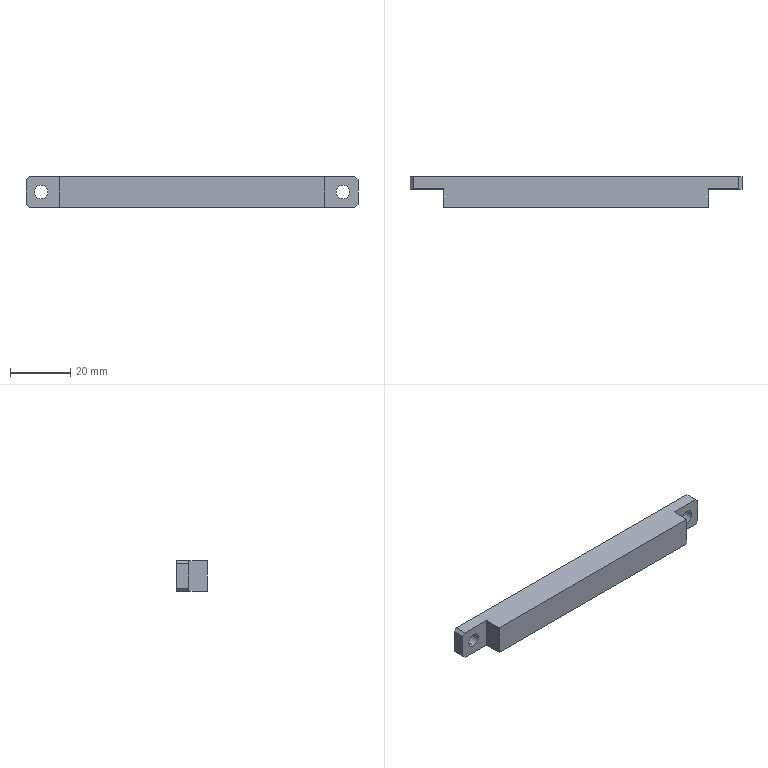Part | STEP file | 08-10 stop block | 1 solid | 18 faces | box 110 x 10 x 10 mm | volume 9545 mm3 | plane 14 | cylinder 4 | commonest cylinder face diameters 4.5 x4
STEP:
#1=CARTESIAN_POINT('',(-50.,-1.5,2.75));
#2=VERTEX_POINT('',#1);
#3=CARTESIAN_POINT('',(-50.,-1.5,7.25));
#4=VERTEX_POINT('',#3);
#5=CARTESIAN_POINT('',(-50.,-1.5,5.));
#6=DIRECTION('',(0.,1.,0.));
#7=DIRECTION('',(-1.,0.,0.));
#8=AXIS2_PLACEMENT_3D('',#5,#6,#7);
#9=CIRCLE('',#8,2.25);
#10=EDGE_CURVE('',#2,#4,#9,.T.);
#11=ORIENTED_EDGE('',*,*,#10,.F.);
#12=CARTESIAN_POINT('',(-50.,2.5,2.75));
#13=VERTEX_POINT('',#12);
#14=CARTESIAN_POINT('',(-50.,7.5,2.75));
#15=DIRECTION('',(0.,1.,0.));
#16=VECTOR('',#15,1000.);
#17=LINE('',#14,#16);
#18=EDGE_CURVE('',#2,#13,#17,.T.);
#19=ORIENTED_EDGE('',*,*,#18,.T.);
#20=CARTESIAN_POINT('',(-50.,2.5,7.25));
#21=VERTEX_POINT('',#20);
#22=CARTESIAN_POINT('',(-50.,2.5,5.));
#23=DIRECTION('',(0.,1.,0.));
#24=DIRECTION('',(0.,0.,-1.));
#25=AXIS2_PLACEMENT_3D('',#22,#23,#24);
#26=CIRCLE('',#25,2.25);
#27=EDGE_CURVE('',#13,#21,#26,.T.);
#28=ORIENTED_EDGE('',*,*,#27,.T.);
#29=CARTESIAN_POINT('',(-50.,7.5,7.25));
#30=DIRECTION('',(0.,1.,0.));
#31=VECTOR('',#30,1000.);
#32=LINE('',#29,#31);
#33=EDGE_CURVE('',#4,#21,#32,.T.);
#34=ORIENTED_EDGE('',*,*,#33,.F.);
#35=EDGE_LOOP('',(#11,#19,#28,#34));
#36=FACE_OUTER_BOUND('',#35,.T.);
#37=CARTESIAN_POINT('',(-50.,7.5,5.));
#38=DIRECTION('',(0.,1.,0.));
#39=DIRECTION('',(0.,0.,1.));
#40=AXIS2_PLACEMENT_3D('',#37,#38,#39);
#41=CYLINDRICAL_SURFACE('',#40,2.25);
#42=ADVANCED_FACE('',(#36),#41,.F.);
#43=CARTESIAN_POINT('',(50.,-1.5,2.75));
#44=VERTEX_POINT('',#43);
#45=CARTESIAN_POINT('',(50.,-1.5,7.25));
#46=VERTEX_POINT('',#45);
#47=CARTESIAN_POINT('',(50.,-1.5,5.));
#48=DIRECTION('',(0.,1.,0.));
#49=DIRECTION('',(-1.,0.,0.));
#50=AXIS2_PLACEMENT_3D('',#47,#48,#49);
#51=CIRCLE('',#50,2.25);
#52=EDGE_CURVE('',#44,#46,#51,.T.);
#53=ORIENTED_EDGE('',*,*,#52,.F.);
#54=CARTESIAN_POINT('',(50.,2.5,2.75));
#55=VERTEX_POINT('',#54);
#56=CARTESIAN_POINT('',(50.,7.5,2.75));
#57=DIRECTION('',(0.,1.,0.));
#58=VECTOR('',#57,1000.);
#59=LINE('',#56,#58);
#60=EDGE_CURVE('',#44,#55,#59,.T.);
#61=ORIENTED_EDGE('',*,*,#60,.T.);
#62=CARTESIAN_POINT('',(50.,2.5,7.25));
#63=VERTEX_POINT('',#62);
#64=CARTESIAN_POINT('',(50.,2.5,5.));
#65=DIRECTION('',(0.,1.,0.));
#66=DIRECTION('',(0.,0.,-1.));
#67=AXIS2_PLACEMENT_3D('',#64,#65,#66);
#68=CIRCLE('',#67,2.25);
#69=EDGE_CURVE('',#55,#63,#68,.T.);
#70=ORIENTED_EDGE('',*,*,#69,.T.);
#71=CARTESIAN_POINT('',(50.,7.5,7.25));
#72=DIRECTION('',(0.,1.,0.));
#73=VECTOR('',#72,1000.);
#74=LINE('',#71,#73);
#75=EDGE_CURVE('',#46,#63,#74,.T.);
#76=ORIENTED_EDGE('',*,*,#75,.F.);
#77=EDGE_LOOP('',(#53,#61,#70,#76));
#78=FACE_OUTER_BOUND('',#77,.T.);
#79=CARTESIAN_POINT('',(50.,7.5,5.));
#80=DIRECTION('',(0.,1.,0.));
#81=DIRECTION('',(0.,0.,1.));
#82=AXIS2_PLACEMENT_3D('',#79,#80,#81);
#83=CYLINDRICAL_SURFACE('',#82,2.25);
#84=ADVANCED_FACE('',(#78),#83,.F.);
#85=CARTESIAN_POINT('',(55.,-1.5,1.));
#86=VERTEX_POINT('',#85);
#87=CARTESIAN_POINT('',(55.,2.5,1.));
#88=VERTEX_POINT('',#87);
#89=CARTESIAN_POINT('',(55.,7.5,1.));
#90=DIRECTION('',(0.,1.,0.));
#91=VECTOR('',#90,1000.);
#92=LINE('',#89,#91);
#93=EDGE_CURVE('',#86,#88,#92,.T.);
#94=ORIENTED_EDGE('',*,*,#93,.T.);
#95=CARTESIAN_POINT('',(55.,2.5,9.));
#96=VERTEX_POINT('',#95);
#97=CARTESIAN_POINT('',(55.,2.5,10.));
#98=DIRECTION('',(0.,0.,1.));
#99=VECTOR('',#98,1000.);
#100=LINE('',#97,#99);
#101=EDGE_CURVE('',#88,#96,#100,.T.);
#102=ORIENTED_EDGE('',*,*,#101,.T.);
#103=CARTESIAN_POINT('',(55.,-1.5,9.));
#104=VERTEX_POINT('',#103);
#105=CARTESIAN_POINT('',(55.,-1.5,9.));
#106=DIRECTION('',(0.,-1.,0.));
#107=VECTOR('',#106,1000.);
#108=LINE('',#105,#107);
#109=EDGE_CURVE('',#96,#104,#108,.T.);
#110=ORIENTED_EDGE('',*,*,#109,.T.);
#111=CARTESIAN_POINT('',(55.,-1.5,0.));
#112=DIRECTION('',(0.,0.,1.));
#113=VECTOR('',#112,1000.);
#114=LINE('',#111,#113);
#115=EDGE_CURVE('',#86,#104,#114,.T.);
#116=ORIENTED_EDGE('',*,*,#115,.F.);
#117=EDGE_LOOP('',(#94,#102,#110,#116));
#118=FACE_OUTER_BOUND('',#117,.T.);
#119=CARTESIAN_POINT('',(55.,7.5,10.));
#120=DIRECTION('',(-1.,0.,0.));
#121=DIRECTION('',(0.,0.,1.));
#122=AXIS2_PLACEMENT_3D('',#119,#120,#121);
#123=PLANE('',#122);
#124=ADVANCED_FACE('',(#118),#123,.F.);
#125=CARTESIAN_POINT('',(-55.,-1.5,9.));
#126=VERTEX_POINT('',#125);
#127=CARTESIAN_POINT('',(-55.,2.5,9.));
#128=VERTEX_POINT('',#127);
#129=CARTESIAN_POINT('',(-55.,7.5,9.));
#130=DIRECTION('',(0.,1.,0.));
#131=VECTOR('',#130,1000.);
#132=LINE('',#129,#131);
#133=EDGE_CURVE('',#126,#128,#132,.T.);
#134=ORIENTED_EDGE('',*,*,#133,.T.);
#135=CARTESIAN_POINT('',(-55.,2.5,1.));
#136=VERTEX_POINT('',#135);
#137=CARTESIAN_POINT('',(-55.,2.5,10.));
#138=DIRECTION('',(0.,0.,-1.));
#139=VECTOR('',#138,1000.);
#140=LINE('',#137,#139);
#141=EDGE_CURVE('',#128,#136,#140,.T.);
#142=ORIENTED_EDGE('',*,*,#141,.T.);
#143=CARTESIAN_POINT('',(-55.,-1.5,1.));
#144=VERTEX_POINT('',#143);
#145=CARTESIAN_POINT('',(-55.,7.5,1.));
#146=DIRECTION('',(0.,-1.,0.));
#147=VECTOR('',#146,1000.);
#148=LINE('',#145,#147);
#149=EDGE_CURVE('',#136,#144,#148,.T.);
#150=ORIENTED_EDGE('',*,*,#149,.T.);
#151=CARTESIAN_POINT('',(-55.,-1.5,0.));
#152=DIRECTION('',(0.,0.,1.));
#153=VECTOR('',#152,1000.);
#154=LINE('',#151,#153);
#155=EDGE_CURVE('',#144,#126,#154,.T.);
#156=ORIENTED_EDGE('',*,*,#155,.T.);
#157=EDGE_LOOP('',(#134,#142,#150,#156));
#158=FACE_OUTER_BOUND('',#157,.T.);
#159=CARTESIAN_POINT('',(-55.,7.5,10.));
#160=DIRECTION('',(1.,0.,0.));
#161=DIRECTION('',(0.,0.,-1.));
#162=AXIS2_PLACEMENT_3D('',#159,#160,#161);
#163=PLANE('',#162);
#164=ADVANCED_FACE('',(#158),#163,.F.);
#165=CARTESIAN_POINT('',(-44.,-7.5,10.));
#166=VERTEX_POINT('',#165);
#167=CARTESIAN_POINT('',(44.,-7.5,10.));
#168=VERTEX_POINT('',#167);
#169=CARTESIAN_POINT('',(-55.,-7.5,10.));
#170=DIRECTION('',(1.,0.,0.));
#171=VECTOR('',#170,1000.);
#172=LINE('',#169,#171);
#173=EDGE_CURVE('',#166,#168,#172,.T.);
#174=ORIENTED_EDGE('',*,*,#173,.F.);
#175=CARTESIAN_POINT('',(-44.,-7.5,0.));
#176=VERTEX_POINT('',#175);
#177=CARTESIAN_POINT('',(-44.,-7.5,0.));
#178=DIRECTION('',(0.,0.,1.));
#179=VECTOR('',#178,1000.);
#180=LINE('',#177,#179);
#181=EDGE_CURVE('',#176,#166,#180,.T.);
#182=ORIENTED_EDGE('',*,*,#181,.F.);
#183=CARTESIAN_POINT('',(44.,-7.5,0.));
#184=VERTEX_POINT('',#183);
#185=CARTESIAN_POINT('',(-55.,-7.5,0.));
#186=DIRECTION('',(1.,0.,0.));
#187=VECTOR('',#186,1000.);
#188=LINE('',#185,#187);
#189=EDGE_CURVE('',#176,#184,#188,.T.);
#190=ORIENTED_EDGE('',*,*,#189,.T.);
#191=CARTESIAN_POINT('',(44.,-7.5,0.));
#192=DIRECTION('',(0.,0.,1.));
#193=VECTOR('',#192,1000.);
#194=LINE('',#191,#193);
#195=EDGE_CURVE('',#184,#168,#194,.T.);
#196=ORIENTED_EDGE('',*,*,#195,.T.);
#197=EDGE_LOOP('',(#174,#182,#190,#196));
#198=FACE_OUTER_BOUND('',#197,.T.);
#199=CARTESIAN_POINT('',(-55.,-7.5,10.));
#200=DIRECTION('',(0.,1.,0.));
#201=DIRECTION('',(0.,0.,1.));
#202=AXIS2_PLACEMENT_3D('',#199,#200,#201);
#203=PLANE('',#202);
#204=ADVANCED_FACE('',(#198),#203,.F.);
#205=CARTESIAN_POINT('',(54.,2.5,10.));
#206=VERTEX_POINT('',#205);
#207=CARTESIAN_POINT('',(-54.,2.5,10.));
#208=VERTEX_POINT('',#207);
#209=CARTESIAN_POINT('',(64.192,2.5,10.));
#210=DIRECTION('',(-1.,0.,0.));
#211=VECTOR('',#210,1000.);
#212=LINE('',#209,#211);
#213=EDGE_CURVE('',#206,#208,#212,.T.);
#214=ORIENTED_EDGE('',*,*,#213,.T.);
#215=CARTESIAN_POINT('',(-54.,-1.5,10.));
#216=VERTEX_POINT('',#215);
#217=CARTESIAN_POINT('',(-54.,-1.5,10.));
#218=DIRECTION('',(0.,-1.,0.));
#219=VECTOR('',#218,1000.);
#220=LINE('',#217,#219);
#221=EDGE_CURVE('',#208,#216,#220,.T.);
#222=ORIENTED_EDGE('',*,*,#221,.T.);
#223=CARTESIAN_POINT('',(-44.,-1.5,10.));
#224=VERTEX_POINT('',#223);
#225=CARTESIAN_POINT('',(-55.,-1.5,10.));
#226=DIRECTION('',(-1.,0.,0.));
#227=VECTOR('',#226,1000.);
#228=LINE('',#225,#227);
#229=EDGE_CURVE('',#224,#216,#228,.T.);
#230=ORIENTED_EDGE('',*,*,#229,.F.);
#231=CARTESIAN_POINT('',(-44.,-7.5,10.));
#232=DIRECTION('',(0.,1.,0.));
#233=VECTOR('',#232,1000.);
#234=LINE('',#231,#233);
#235=EDGE_CURVE('',#166,#224,#234,.T.);
#236=ORIENTED_EDGE('',*,*,#235,.F.);
#237=ORIENTED_EDGE('',*,*,#173,.T.);
#238=CARTESIAN_POINT('',(44.,-1.5,10.));
#239=VERTEX_POINT('',#238);
#240=CARTESIAN_POINT('',(44.,-7.5,10.));
#241=DIRECTION('',(0.,-1.,0.));
#242=VECTOR('',#241,1000.);
#243=LINE('',#240,#242);
#244=EDGE_CURVE('',#239,#168,#243,.T.);
#245=ORIENTED_EDGE('',*,*,#244,.F.);
#246=CARTESIAN_POINT('',(54.,-1.5,10.));
#247=VERTEX_POINT('',#246);
#248=CARTESIAN_POINT('',(55.,-1.5,10.));
#249=DIRECTION('',(-1.,0.,0.));
#250=VECTOR('',#249,1000.);
#251=LINE('',#248,#250);
#252=EDGE_CURVE('',#247,#239,#251,.T.);
#253=ORIENTED_EDGE('',*,*,#252,.F.);
#254=CARTESIAN_POINT('',(54.,7.5,10.));
#255=DIRECTION('',(0.,1.,0.));
#256=VECTOR('',#255,1000.);
#257=LINE('',#254,#256);
#258=EDGE_CURVE('',#247,#206,#257,.T.);
#259=ORIENTED_EDGE('',*,*,#258,.T.);
#260=EDGE_LOOP('',(#214,#222,#230,#236,#237,#245,#253,#259));
#261=FACE_OUTER_BOUND('',#260,.T.);
#262=CARTESIAN_POINT('',(55.,-7.5,10.));
#263=DIRECTION('',(0.,0.,1.));
#264=DIRECTION('',(1.,0.,0.));
#265=AXIS2_PLACEMENT_3D('',#262,#263,#264);
#266=PLANE('',#265);
#267=ADVANCED_FACE('',(#261),#266,.T.);
#268=CARTESIAN_POINT('',(-54.,-1.5,0.));
#269=VERTEX_POINT('',#268);
#270=CARTESIAN_POINT('',(-54.,2.5,0.));
#271=VERTEX_POINT('',#270);
#272=CARTESIAN_POINT('',(-54.,-7.5,0.));
#273=DIRECTION('',(0.,1.,0.));
#274=VECTOR('',#273,1000.);
#275=LINE('',#272,#274);
#276=EDGE_CURVE('',#269,#271,#275,.T.);
#277=ORIENTED_EDGE('',*,*,#276,.T.);
#278=CARTESIAN_POINT('',(54.,2.5,0.));
#279=VERTEX_POINT('',#278);
#280=CARTESIAN_POINT('',(64.192,2.5,0.));
#281=DIRECTION('',(-1.,0.,0.));
#282=VECTOR('',#281,1000.);
#283=LINE('',#280,#282);
#284=EDGE_CURVE('',#279,#271,#283,.T.);
#285=ORIENTED_EDGE('',*,*,#284,.F.);
#286=CARTESIAN_POINT('',(54.,-1.5,0.));
#287=VERTEX_POINT('',#286);
#288=CARTESIAN_POINT('',(54.,-7.5,0.));
#289=DIRECTION('',(0.,-1.,0.));
#290=VECTOR('',#289,1000.);
#291=LINE('',#288,#290);
#292=EDGE_CURVE('',#279,#287,#291,.T.);
#293=ORIENTED_EDGE('',*,*,#292,.T.);
#294=CARTESIAN_POINT('',(44.,-1.5,0.));
#295=VERTEX_POINT('',#294);
#296=CARTESIAN_POINT('',(55.,-1.5,0.));
#297=DIRECTION('',(-1.,0.,0.));
#298=VECTOR('',#297,1000.);
#299=LINE('',#296,#298);
#300=EDGE_CURVE('',#287,#295,#299,.T.);
#301=ORIENTED_EDGE('',*,*,#300,.T.);
#302=CARTESIAN_POINT('',(44.,-7.5,0.));
#303=DIRECTION('',(0.,-1.,0.));
#304=VECTOR('',#303,1000.);
#305=LINE('',#302,#304);
#306=EDGE_CURVE('',#295,#184,#305,.T.);
#307=ORIENTED_EDGE('',*,*,#306,.T.);
#308=ORIENTED_EDGE('',*,*,#189,.F.);
#309=CARTESIAN_POINT('',(-44.,-1.5,0.));
#310=VERTEX_POINT('',#309);
#311=CARTESIAN_POINT('',(-44.,-7.5,0.));
#312=DIRECTION('',(0.,1.,0.));
#313=VECTOR('',#312,1000.);
#314=LINE('',#311,#313);
#315=EDGE_CURVE('',#176,#310,#314,.T.);
#316=ORIENTED_EDGE('',*,*,#315,.T.);
#317=CARTESIAN_POINT('',(-55.,-1.5,0.));
#318=DIRECTION('',(-1.,0.,0.));
#319=VECTOR('',#318,1000.);
#320=LINE('',#317,#319);
#321=EDGE_CURVE('',#310,#269,#320,.T.);
#322=ORIENTED_EDGE('',*,*,#321,.T.);
#323=EDGE_LOOP('',(#277,#285,#293,#301,#307,#308,#316,#322));
#324=FACE_OUTER_BOUND('',#323,.T.);
#325=CARTESIAN_POINT('',(55.,-7.5,0.));
#326=DIRECTION('',(0.,0.,1.));
#327=DIRECTION('',(1.,0.,0.));
#328=AXIS2_PLACEMENT_3D('',#325,#326,#327);
#329=PLANE('',#328);
#330=ADVANCED_FACE('',(#324),#329,.F.);
#331=ORIENTED_EDGE('',*,*,#244,.T.);
#332=ORIENTED_EDGE('',*,*,#195,.F.);
#333=ORIENTED_EDGE('',*,*,#306,.F.);
#334=CARTESIAN_POINT('',(44.,-1.5,0.));
#335=DIRECTION('',(0.,0.,1.));
#336=VECTOR('',#335,1000.);
#337=LINE('',#334,#336);
#338=EDGE_CURVE('',#295,#239,#337,.T.);
#339=ORIENTED_EDGE('',*,*,#338,.T.);
#340=EDGE_LOOP('',(#331,#332,#333,#339));
#341=FACE_OUTER_BOUND('',#340,.T.);
#342=CARTESIAN_POINT('',(44.,-7.5,0.));
#343=DIRECTION('',(-1.,0.,0.));
#344=DIRECTION('',(0.,0.,1.));
#345=AXIS2_PLACEMENT_3D('',#342,#343,#344);
#346=PLANE('',#345);
#347=ADVANCED_FACE('',(#341),#346,.F.);
#348=CARTESIAN_POINT('',(50.,-1.5,5.));
#349=DIRECTION('',(0.,1.,0.));
#350=DIRECTION('',(-1.,0.,0.));
#351=AXIS2_PLACEMENT_3D('',#348,#349,#350);
#352=CIRCLE('',#351,2.25);
#353=EDGE_CURVE('',#46,#44,#352,.T.);
#354=ORIENTED_EDGE('',*,*,#353,.T.);
#355=ORIENTED_EDGE('',*,*,#52,.T.);
#356=EDGE_LOOP('',(#354,#355));
#357=FACE_BOUND('',#356,.T.);
#358=ORIENTED_EDGE('',*,*,#300,.F.);
#359=CARTESIAN_POINT('',(55.,-1.5,1.));
#360=DIRECTION('',(0.7071,0.,0.7071));
#361=VECTOR('',#360,1000.);
#362=LINE('',#359,#361);
#363=EDGE_CURVE('',#287,#86,#362,.T.);
#364=ORIENTED_EDGE('',*,*,#363,.T.);
#365=ORIENTED_EDGE('',*,*,#115,.T.);
#366=CARTESIAN_POINT('',(54.,-1.5,10.));
#367=DIRECTION('',(-0.7071,0.,0.7071));
#368=VECTOR('',#367,1000.);
#369=LINE('',#366,#368);
#370=EDGE_CURVE('',#104,#247,#369,.T.);
#371=ORIENTED_EDGE('',*,*,#370,.T.);
#372=ORIENTED_EDGE('',*,*,#252,.T.);
#373=ORIENTED_EDGE('',*,*,#338,.F.);
#374=EDGE_LOOP('',(#358,#364,#365,#371,#372,#373));
#375=FACE_OUTER_BOUND('',#374,.T.);
#376=CARTESIAN_POINT('',(55.,-1.5,0.));
#377=DIRECTION('',(0.,1.,0.));
#378=DIRECTION('',(-1.,0.,0.));
#379=AXIS2_PLACEMENT_3D('',#376,#377,#378);
#380=PLANE('',#379);
#381=ADVANCED_FACE('',(#357,#375),#380,.F.);
#382=CARTESIAN_POINT('',(-50.,-1.5,5.));
#383=DIRECTION('',(0.,1.,0.));
#384=DIRECTION('',(-1.,0.,0.));
#385=AXIS2_PLACEMENT_3D('',#382,#383,#384);
#386=CIRCLE('',#385,2.25);
#387=EDGE_CURVE('',#4,#2,#386,.T.);
#388=ORIENTED_EDGE('',*,*,#387,.T.);
#389=ORIENTED_EDGE('',*,*,#10,.T.);
#390=EDGE_LOOP('',(#388,#389));
#391=FACE_BOUND('',#390,.T.);
#392=ORIENTED_EDGE('',*,*,#229,.T.);
#393=CARTESIAN_POINT('',(-54.,-1.5,10.));
#394=DIRECTION('',(-0.7071,0.,-0.7071));
#395=VECTOR('',#394,1000.);
#396=LINE('',#393,#395);
#397=EDGE_CURVE('',#216,#126,#396,.T.);
#398=ORIENTED_EDGE('',*,*,#397,.T.);
#399=ORIENTED_EDGE('',*,*,#155,.F.);
#400=CARTESIAN_POINT('',(-55.,-1.5,1.));
#401=DIRECTION('',(0.7071,0.,-0.7071));
#402=VECTOR('',#401,1000.);
#403=LINE('',#400,#402);
#404=EDGE_CURVE('',#144,#269,#403,.T.);
#405=ORIENTED_EDGE('',*,*,#404,.T.);
#406=ORIENTED_EDGE('',*,*,#321,.F.);
#407=CARTESIAN_POINT('',(-44.,-1.5,0.));
#408=DIRECTION('',(0.,0.,1.));
#409=VECTOR('',#408,1000.);
#410=LINE('',#407,#409);
#411=EDGE_CURVE('',#310,#224,#410,.T.);
#412=ORIENTED_EDGE('',*,*,#411,.T.);
#413=EDGE_LOOP('',(#392,#398,#399,#405,#406,#412));
#414=FACE_OUTER_BOUND('',#413,.T.);
#415=CARTESIAN_POINT('',(-55.,-1.5,0.));
#416=DIRECTION('',(0.,1.,0.));
#417=DIRECTION('',(-1.,0.,0.));
#418=AXIS2_PLACEMENT_3D('',#415,#416,#417);
#419=PLANE('',#418);
#420=ADVANCED_FACE('',(#391,#414),#419,.F.);
#421=ORIENTED_EDGE('',*,*,#235,.T.);
#422=ORIENTED_EDGE('',*,*,#411,.F.);
#423=ORIENTED_EDGE('',*,*,#315,.F.);
#424=ORIENTED_EDGE('',*,*,#181,.T.);
#425=EDGE_LOOP('',(#421,#422,#423,#424));
#426=FACE_OUTER_BOUND('',#425,.T.);
#427=CARTESIAN_POINT('',(-44.,-7.5,0.));
#428=DIRECTION('',(1.,0.,0.));
#429=DIRECTION('',(0.,0.,-1.));
#430=AXIS2_PLACEMENT_3D('',#427,#428,#429);
#431=PLANE('',#430);
#432=ADVANCED_FACE('',(#426),#431,.F.);
#433=ORIENTED_EDGE('',*,*,#60,.F.);
#434=ORIENTED_EDGE('',*,*,#353,.F.);
#435=ORIENTED_EDGE('',*,*,#75,.T.);
#436=CARTESIAN_POINT('',(50.,2.5,5.));
#437=DIRECTION('',(0.,1.,0.));
#438=DIRECTION('',(0.,0.,-1.));
#439=AXIS2_PLACEMENT_3D('',#436,#437,#438);
#440=CIRCLE('',#439,2.25);
#441=EDGE_CURVE('',#63,#55,#440,.T.);
#442=ORIENTED_EDGE('',*,*,#441,.T.);
#443=EDGE_LOOP('',(#433,#434,#435,#442));
#444=FACE_OUTER_BOUND('',#443,.T.);
#445=CARTESIAN_POINT('',(50.,7.5,5.));
#446=DIRECTION('',(0.,1.,0.));
#447=DIRECTION('',(0.,0.,1.));
#448=AXIS2_PLACEMENT_3D('',#445,#446,#447);
#449=CYLINDRICAL_SURFACE('',#448,2.25);
#450=ADVANCED_FACE('',(#444),#449,.F.);
#451=ORIENTED_EDGE('',*,*,#18,.F.);
#452=ORIENTED_EDGE('',*,*,#387,.F.);
#453=ORIENTED_EDGE('',*,*,#33,.T.);
#454=CARTESIAN_POINT('',(-50.,2.5,5.));
#455=DIRECTION('',(0.,1.,0.));
#456=DIRECTION('',(0.,0.,-1.));
#457=AXIS2_PLACEMENT_3D('',#454,#455,#456);
#458=CIRCLE('',#457,2.25);
#459=EDGE_CURVE('',#21,#13,#458,.T.);
#460=ORIENTED_EDGE('',*,*,#459,.T.);
#461=EDGE_LOOP('',(#451,#452,#453,#460));
#462=FACE_OUTER_BOUND('',#461,.T.);
#463=CARTESIAN_POINT('',(-50.,7.5,5.));
#464=DIRECTION('',(0.,1.,0.));
#465=DIRECTION('',(0.,0.,1.));
#466=AXIS2_PLACEMENT_3D('',#463,#464,#465);
#467=CYLINDRICAL_SURFACE('',#466,2.25);
#468=ADVANCED_FACE('',(#462),#467,.F.);
#469=CARTESIAN_POINT('',(-54.,2.5,10.));
#470=DIRECTION('',(0.7071,0.,0.7071));
#471=VECTOR('',#470,1000.);
#472=LINE('',#469,#471);
#473=EDGE_CURVE('',#128,#208,#472,.T.);
#474=ORIENTED_EDGE('',*,*,#473,.F.);
#475=ORIENTED_EDGE('',*,*,#133,.F.);
#476=ORIENTED_EDGE('',*,*,#397,.F.);
#477=ORIENTED_EDGE('',*,*,#221,.F.);
#478=EDGE_LOOP('',(#474,#475,#476,#477));
#479=FACE_OUTER_BOUND('',#478,.T.);
#480=CARTESIAN_POINT('',(-54.,-7.5,10.));
#481=DIRECTION('',(-0.7071,0.,0.7071));
#482=DIRECTION('',(0.7071,0.,0.7071));
#483=AXIS2_PLACEMENT_3D('',#480,#481,#482);
#484=PLANE('',#483);
#485=ADVANCED_FACE('',(#479),#484,.T.);
#486=CARTESIAN_POINT('',(-55.,2.5,1.));
#487=DIRECTION('',(-0.7071,0.,0.7071));
#488=VECTOR('',#487,1000.);
#489=LINE('',#486,#488);
#490=EDGE_CURVE('',#271,#136,#489,.T.);
#491=ORIENTED_EDGE('',*,*,#490,.F.);
#492=ORIENTED_EDGE('',*,*,#276,.F.);
#493=ORIENTED_EDGE('',*,*,#404,.F.);
#494=ORIENTED_EDGE('',*,*,#149,.F.);
#495=EDGE_LOOP('',(#491,#492,#493,#494));
#496=FACE_OUTER_BOUND('',#495,.T.);
#497=CARTESIAN_POINT('',(-55.,7.5,1.));
#498=DIRECTION('',(0.7071,0.,0.7071));
#499=DIRECTION('',(0.7071,0.,-0.7071));
#500=AXIS2_PLACEMENT_3D('',#497,#498,#499);
#501=PLANE('',#500);
#502=ADVANCED_FACE('',(#496),#501,.F.);
#503=CARTESIAN_POINT('',(55.,2.5,1.));
#504=DIRECTION('',(-0.7071,0.,-0.7071));
#505=VECTOR('',#504,1000.);
#506=LINE('',#503,#505);
#507=EDGE_CURVE('',#88,#279,#506,.T.);
#508=ORIENTED_EDGE('',*,*,#507,.F.);
#509=ORIENTED_EDGE('',*,*,#93,.F.);
#510=ORIENTED_EDGE('',*,*,#363,.F.);
#511=ORIENTED_EDGE('',*,*,#292,.F.);
#512=EDGE_LOOP('',(#508,#509,#510,#511));
#513=FACE_OUTER_BOUND('',#512,.T.);
#514=CARTESIAN_POINT('',(55.,7.5,1.));
#515=DIRECTION('',(-0.7071,0.,0.7071));
#516=DIRECTION('',(0.7071,0.,0.7071));
#517=AXIS2_PLACEMENT_3D('',#514,#515,#516);
#518=PLANE('',#517);
#519=ADVANCED_FACE('',(#513),#518,.F.);
#520=CARTESIAN_POINT('',(54.,2.5,10.));
#521=DIRECTION('',(0.7071,0.,-0.7071));
#522=VECTOR('',#521,1000.);
#523=LINE('',#520,#522);
#524=EDGE_CURVE('',#206,#96,#523,.T.);
#525=ORIENTED_EDGE('',*,*,#524,.F.);
#526=ORIENTED_EDGE('',*,*,#258,.F.);
#527=ORIENTED_EDGE('',*,*,#370,.F.);
#528=ORIENTED_EDGE('',*,*,#109,.F.);
#529=EDGE_LOOP('',(#525,#526,#527,#528));
#530=FACE_OUTER_BOUND('',#529,.T.);
#531=CARTESIAN_POINT('',(54.,-7.5,10.));
#532=DIRECTION('',(0.7071,0.,0.7071));
#533=DIRECTION('',(0.7071,0.,-0.7071));
#534=AXIS2_PLACEMENT_3D('',#531,#532,#533);
#535=PLANE('',#534);
#536=ADVANCED_FACE('',(#530),#535,.T.);
#537=ORIENTED_EDGE('',*,*,#459,.F.);
#538=ORIENTED_EDGE('',*,*,#27,.F.);
#539=EDGE_LOOP('',(#537,#538));
#540=FACE_BOUND('',#539,.T.);
#541=ORIENTED_EDGE('',*,*,#473,.T.);
#542=ORIENTED_EDGE('',*,*,#213,.F.);
#543=ORIENTED_EDGE('',*,*,#524,.T.);
#544=ORIENTED_EDGE('',*,*,#101,.F.);
#545=ORIENTED_EDGE('',*,*,#507,.T.);
#546=ORIENTED_EDGE('',*,*,#284,.T.);
#547=ORIENTED_EDGE('',*,*,#490,.T.);
#548=ORIENTED_EDGE('',*,*,#141,.F.);
#549=EDGE_LOOP('',(#541,#542,#543,#544,#545,#546,#547,#548));
#550=FACE_OUTER_BOUND('',#549,.T.);
#551=ORIENTED_EDGE('',*,*,#441,.F.);
#552=ORIENTED_EDGE('',*,*,#69,.F.);
#553=EDGE_LOOP('',(#551,#552));
#554=FACE_BOUND('',#553,.T.);
#555=CARTESIAN_POINT('',(64.192,2.5,10.));
#556=DIRECTION('',(0.,-1.,0.));
#557=DIRECTION('',(0.,0.,-1.));
#558=AXIS2_PLACEMENT_3D('',#555,#556,#557);
#559=PLANE('',#558);
#560=ADVANCED_FACE('',(#540,#550,#554),#559,.F.);
#561=CLOSED_SHELL('',(#42,#84,#124,#164,#204,#267,#330,#347,#381,#420,#432,#450,#468,#485,#502,#519,#536,#560));
#562=MANIFOLD_SOLID_BREP('',#561);
#563=CARTESIAN_POINT('',(0.,0.,0.));
#564=DIRECTION('',(0.,0.,1.));
#565=DIRECTION('',(1.,0.,0.));
#566=AXIS2_PLACEMENT_3D('',#563,#564,#565);
#567=(LENGTH_UNIT()NAMED_UNIT(*)SI_UNIT(.MILLI.,.METRE.));
#568=UNCERTAINTY_MEASURE_WITH_UNIT(LENGTH_MEASURE(0.00001),#567,'','');
#569=(NAMED_UNIT(*)PLANE_ANGLE_UNIT()SI_UNIT($,.RADIAN.));
#570=(NAMED_UNIT(*)SI_UNIT($,.STERADIAN.)SOLID_ANGLE_UNIT());
#571=(GEOMETRIC_REPRESENTATION_CONTEXT(3)GLOBAL_UNCERTAINTY_ASSIGNED_CONTEXT((#568))GLOBAL_UNIT_ASSIGNED_CONTEXT((#567,#569,#570))REPRESENTATION_CONTEXT('',''));
#572=ADVANCED_BREP_SHAPE_REPRESENTATION('',(#562,#566),#571);